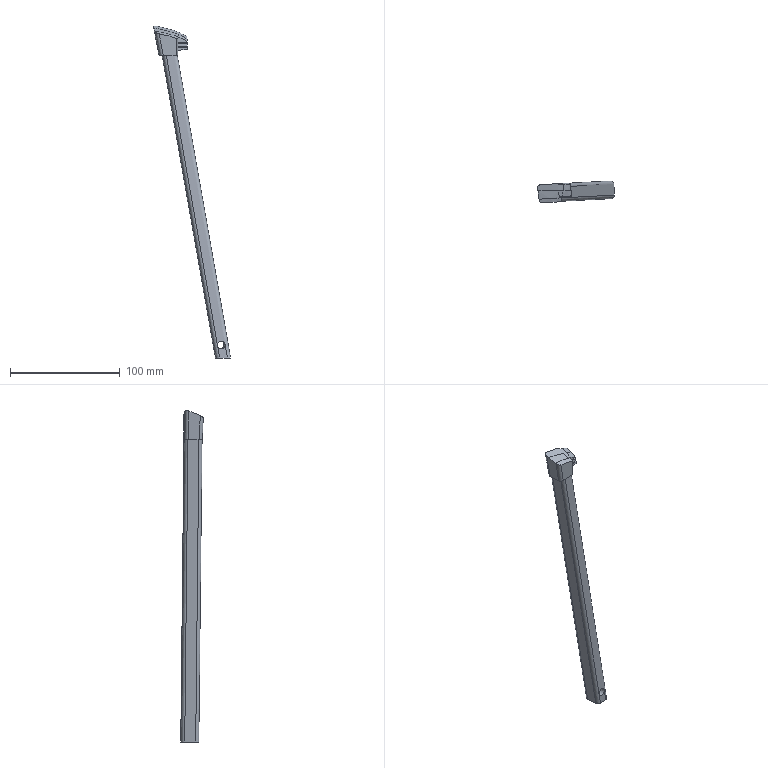Part | STEP file | 车灯-后视镜_id678_x_t | 1 solid | 53 faces | box 70.106 x 20.475 x 302.011 mm | volume 62813 mm3 | plane 32 | spline 13 | cylinder 8 | commonest cylinder face diameters 6 x6 2 x1 7 x1